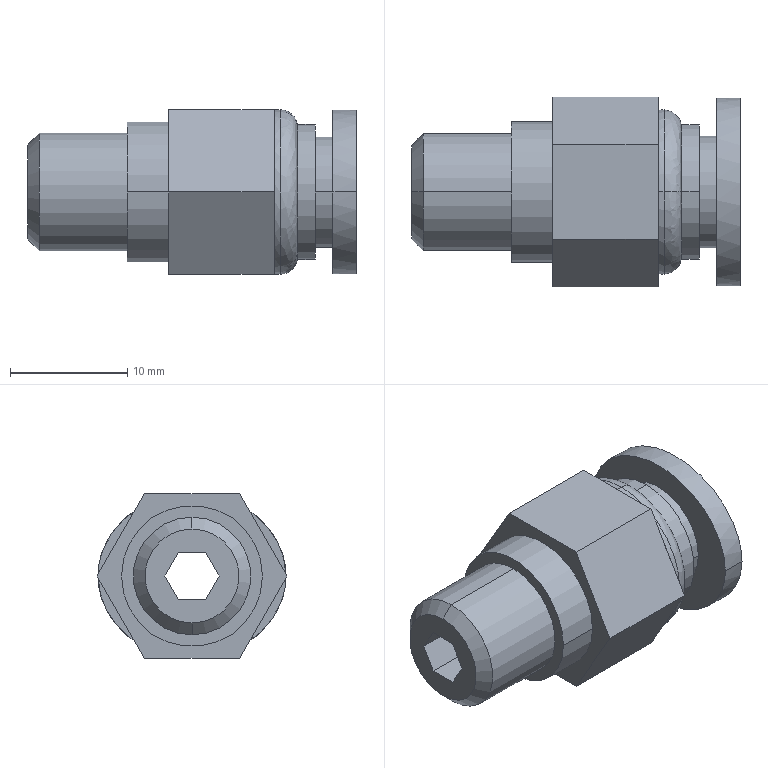Part | STEP file | 1/8 Φ8 fitting | 1 solid | 44 faces | box 28 x 16.166 x 14 mm | volume 2653 mm3 | plane 26 | cylinder 12 | spline 4 | cone 2 | commonest cylinder face diameters 8 x2 9.5 x2 10 x2 11.5 x2 12 x2 14 x2